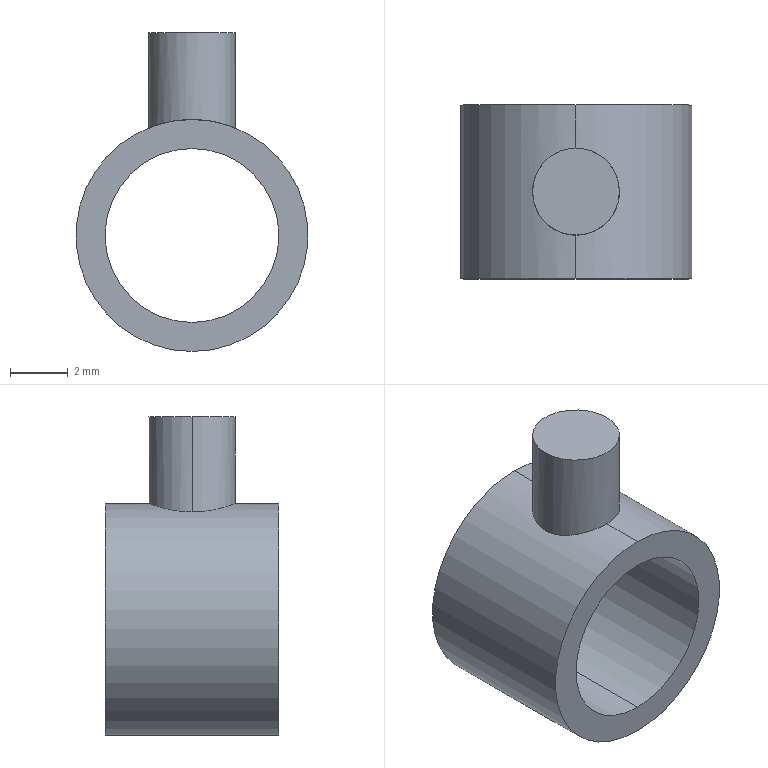Part | SolidWorks | features Extrusion 1, ICE 1 | 1 solid | 9 faces | box 8 x 6 x 11 mm | volume 153.659 mm3 | cylinder 6 | plane 3 | commonest cylinder face diameters 3 x2 6 x2 8 x2
STEP:
#1=CARTESIAN_POINT('',(0.,4.5,4.));
#2=VERTEX_POINT('',#1);
#3=CARTESIAN_POINT('',(-1.5,3.,3.708));
#4=VERTEX_POINT('',#3);
#5=CARTESIAN_POINT('',(0.,4.5,4.));
#6=CARTESIAN_POINT('',(-0.09889,4.5,4.));
#7=CARTESIAN_POINT('',(-0.1992,4.49,3.996));
#8=CARTESIAN_POINT('',(-0.3924,4.451,3.982));
#9=CARTESIAN_POINT('',(-0.4864,4.422,3.971));
#10=CARTESIAN_POINT('',(-0.6693,4.346,3.945));
#11=CARTESIAN_POINT('',(-0.7553,4.3,3.929));
#12=CARTESIAN_POINT('',(-0.9168,4.191,3.894));
#13=CARTESIAN_POINT('',(-0.9931,4.128,3.875));
#14=CARTESIAN_POINT('',(-1.131,3.991,3.838));
#15=CARTESIAN_POINT('',(-1.192,3.916,3.819));
#16=CARTESIAN_POINT('',(-1.3,3.754,3.783));
#17=CARTESIAN_POINT('',(-1.347,3.666,3.766));
#18=CARTESIAN_POINT('',(-1.46,3.396,3.725));
#19=CARTESIAN_POINT('',(-1.5,3.197,3.708));
#20=CARTESIAN_POINT('',(-1.5,3.,3.708));
#21=B_SPLINE_CURVE_WITH_KNOTS('',3,(#5,#6,#7,#8,#9,#10,#11,#12,#13,#14,#15,#16,#17,#18,#19,#20),.UNSPECIFIED.,.F.,.F.,(4,2,2,2,2,2,2,4),(0.002367,0.002663,0.002959,0.003255,0.00355,0.003846,0.004142,0.004733),.UNSPECIFIED.);
#22=EDGE_CURVE('',#2,#4,#21,.T.);
#23=ORIENTED_EDGE('',*,*,#22,.T.);
#24=CARTESIAN_POINT('',(-1.5,3.,7.));
#25=VERTEX_POINT('',#24);
#26=CARTESIAN_POINT('',(-1.5,3.,-4.001));
#27=DIRECTION('',(0.,0.,1.));
#28=VECTOR('',#27,1000.);
#29=LINE('',#26,#28);
#30=EDGE_CURVE('',#4,#25,#29,.T.);
#31=ORIENTED_EDGE('',*,*,#30,.T.);
#32=CARTESIAN_POINT('',(1.5,3.,7.));
#33=VERTEX_POINT('',#32);
#34=CARTESIAN_POINT('',(0.,3.,7.));
#35=DIRECTION('',(0.,0.,1.));
#36=DIRECTION('',(1.,0.,0.));
#37=AXIS2_PLACEMENT_3D('',#34,#35,#36);
#38=CIRCLE('',#37,1.5);
#39=EDGE_CURVE('',#33,#25,#38,.T.);
#40=ORIENTED_EDGE('',*,*,#39,.F.);
#41=CARTESIAN_POINT('',(1.5,3.,3.708));
#42=VERTEX_POINT('',#41);
#43=CARTESIAN_POINT('',(1.5,3.,-4.001));
#44=DIRECTION('',(0.,0.,1.));
#45=VECTOR('',#44,1000.);
#46=LINE('',#43,#45);
#47=EDGE_CURVE('',#42,#33,#46,.T.);
#48=ORIENTED_EDGE('',*,*,#47,.F.);
#49=CARTESIAN_POINT('',(1.5,3.,3.708));
#50=CARTESIAN_POINT('',(1.5,3.1,3.708));
#51=CARTESIAN_POINT('',(1.49,3.198,3.712));
#52=CARTESIAN_POINT('',(1.451,3.391,3.727));
#53=CARTESIAN_POINT('',(1.422,3.487,3.739));
#54=CARTESIAN_POINT('',(1.309,3.759,3.781));
#55=CARTESIAN_POINT('',(1.197,3.924,3.819));
#56=CARTESIAN_POINT('',(0.9232,4.198,3.895));
#57=CARTESIAN_POINT('',(0.7573,4.309,3.932));
#58=CARTESIAN_POINT('',(0.4867,4.422,3.971));
#59=CARTESIAN_POINT('',(0.3912,4.451,3.982));
#60=CARTESIAN_POINT('',(0.197,4.49,3.996));
#61=CARTESIAN_POINT('',(0.09895,4.5,4.));
#62=CARTESIAN_POINT('',(0.,4.5,4.));
#63=B_SPLINE_CURVE_WITH_KNOTS('',3,(#49,#50,#51,#52,#53,#54,#55,#56,#57,#58,#59,#60,#61,#62),.UNSPECIFIED.,.F.,.F.,(4,2,2,2,2,2,4),(0.,0.0002959,0.0005918,0.001184,0.001775,0.002071,0.002367),.UNSPECIFIED.);
#64=EDGE_CURVE('',#42,#2,#63,.T.);
#65=ORIENTED_EDGE('',*,*,#64,.T.);
#66=EDGE_LOOP('',(#23,#31,#40,#48,#65));
#67=FACE_OUTER_BOUND('',#66,.T.);
#68=CARTESIAN_POINT('',(0.,3.,-4.001));
#69=DIRECTION('',(0.,0.,1.));
#70=DIRECTION('',(1.,0.,0.));
#71=AXIS2_PLACEMENT_3D('',#68,#69,#70);
#72=CYLINDRICAL_SURFACE('',#71,1.5);
#73=ADVANCED_FACE('',(#67),#72,.T.);
#74=CARTESIAN_POINT('',(0.,6.,-3.));
#75=VERTEX_POINT('',#74);
#76=CARTESIAN_POINT('',(0.,6.,3.));
#77=VERTEX_POINT('',#76);
#78=CARTESIAN_POINT('',(0.,6.,0.));
#79=DIRECTION('',(0.,1.,0.));
#80=DIRECTION('',(0.,0.,1.));
#81=AXIS2_PLACEMENT_3D('',#78,#79,#80);
#82=CIRCLE('',#81,3.);
#83=EDGE_CURVE('',#75,#77,#82,.T.);
#84=ORIENTED_EDGE('',*,*,#83,.T.);
#85=CARTESIAN_POINT('',(0.,0.,3.));
#86=VERTEX_POINT('',#85);
#87=CARTESIAN_POINT('',(0.,6.,3.));
#88=DIRECTION('',(0.,-1.,0.));
#89=VECTOR('',#88,1000.);
#90=LINE('',#87,#89);
#91=EDGE_CURVE('',#77,#86,#90,.T.);
#92=ORIENTED_EDGE('',*,*,#91,.T.);
#93=CARTESIAN_POINT('',(0.,0.,-3.));
#94=VERTEX_POINT('',#93);
#95=CARTESIAN_POINT('',(0.,0.,0.));
#96=DIRECTION('',(0.,1.,0.));
#97=DIRECTION('',(0.,0.,1.));
#98=AXIS2_PLACEMENT_3D('',#95,#96,#97);
#99=CIRCLE('',#98,3.);
#100=EDGE_CURVE('',#94,#86,#99,.T.);
#101=ORIENTED_EDGE('',*,*,#100,.F.);
#102=CARTESIAN_POINT('',(0.,6.,-3.));
#103=DIRECTION('',(0.,-1.,0.));
#104=VECTOR('',#103,1000.);
#105=LINE('',#102,#104);
#106=EDGE_CURVE('',#75,#94,#105,.T.);
#107=ORIENTED_EDGE('',*,*,#106,.F.);
#108=EDGE_LOOP('',(#84,#92,#101,#107));
#109=FACE_OUTER_BOUND('',#108,.T.);
#110=CARTESIAN_POINT('',(0.,6.,0.));
#111=DIRECTION('',(0.,-1.,0.));
#112=DIRECTION('',(0.,0.,-1.));
#113=AXIS2_PLACEMENT_3D('',#110,#111,#112);
#114=CYLINDRICAL_SURFACE('',#113,3.);
#115=ADVANCED_FACE('',(#109),#114,.F.);
#116=CARTESIAN_POINT('',(0.,6.,4.));
#117=VERTEX_POINT('',#116);
#118=CARTESIAN_POINT('',(0.,6.,-4.));
#119=VERTEX_POINT('',#118);
#120=CARTESIAN_POINT('',(0.,6.,0.));
#121=DIRECTION('',(0.,1.,0.));
#122=DIRECTION('',(0.,0.,1.));
#123=AXIS2_PLACEMENT_3D('',#120,#121,#122);
#124=CIRCLE('',#123,4.);
#125=EDGE_CURVE('',#117,#119,#124,.T.);
#126=ORIENTED_EDGE('',*,*,#125,.F.);
#127=CARTESIAN_POINT('',(0.,6.,4.));
#128=DIRECTION('',(0.,-1.,0.));
#129=VECTOR('',#128,1000.);
#130=LINE('',#127,#129);
#131=EDGE_CURVE('',#117,#2,#130,.T.);
#132=ORIENTED_EDGE('',*,*,#131,.T.);
#133=ORIENTED_EDGE('',*,*,#64,.F.);
#134=CARTESIAN_POINT('',(0.,1.5,4.));
#135=VERTEX_POINT('',#134);
#136=CARTESIAN_POINT('',(0.,1.5,4.));
#137=CARTESIAN_POINT('',(0.1978,1.5,4.));
#138=CARTESIAN_POINT('',(0.3966,1.54,3.984));
#139=CARTESIAN_POINT('',(0.7582,1.691,3.932));
#140=CARTESIAN_POINT('',(0.9237,1.802,3.895));
#141=CARTESIAN_POINT('',(1.13,2.009,3.838));
#142=CARTESIAN_POINT('',(1.193,2.085,3.818));
#143=CARTESIAN_POINT('',(1.301,2.247,3.783));
#144=CARTESIAN_POINT('',(1.347,2.332,3.767));
#145=CARTESIAN_POINT('',(1.461,2.605,3.725));
#146=CARTESIAN_POINT('',(1.5,2.8,3.708));
#147=CARTESIAN_POINT('',(1.5,3.,3.708));
#148=B_SPLINE_CURVE_WITH_KNOTS('',3,(#136,#137,#138,#139,#140,#141,#142,#143,#144,#145,#146,#147),.UNSPECIFIED.,.F.,.F.,(4,2,2,2,2,4),(0.007099,0.00769,0.008282,0.008578,0.008874,0.009465),.UNSPECIFIED.);
#149=EDGE_CURVE('',#135,#42,#148,.T.);
#150=ORIENTED_EDGE('',*,*,#149,.F.);
#151=CARTESIAN_POINT('',(0.,0.,4.));
#152=VERTEX_POINT('',#151);
#153=CARTESIAN_POINT('',(0.,6.,4.));
#154=DIRECTION('',(0.,-1.,0.));
#155=VECTOR('',#154,1000.);
#156=LINE('',#153,#155);
#157=EDGE_CURVE('',#135,#152,#156,.T.);
#158=ORIENTED_EDGE('',*,*,#157,.T.);
#159=CARTESIAN_POINT('',(0.,0.,-4.));
#160=VERTEX_POINT('',#159);
#161=CARTESIAN_POINT('',(0.,0.,0.));
#162=DIRECTION('',(0.,1.,0.));
#163=DIRECTION('',(0.,0.,1.));
#164=AXIS2_PLACEMENT_3D('',#161,#162,#163);
#165=CIRCLE('',#164,4.);
#166=EDGE_CURVE('',#152,#160,#165,.T.);
#167=ORIENTED_EDGE('',*,*,#166,.T.);
#168=CARTESIAN_POINT('',(0.,6.,-4.));
#169=DIRECTION('',(0.,-1.,0.));
#170=VECTOR('',#169,1000.);
#171=LINE('',#168,#170);
#172=EDGE_CURVE('',#119,#160,#171,.T.);
#173=ORIENTED_EDGE('',*,*,#172,.F.);
#174=EDGE_LOOP('',(#126,#132,#133,#150,#158,#167,#173));
#175=FACE_OUTER_BOUND('',#174,.T.);
#176=CARTESIAN_POINT('',(0.,6.,0.));
#177=DIRECTION('',(0.,-1.,0.));
#178=DIRECTION('',(0.,0.,-1.));
#179=AXIS2_PLACEMENT_3D('',#176,#177,#178);
#180=CYLINDRICAL_SURFACE('',#179,4.);
#181=ADVANCED_FACE('',(#175),#180,.T.);
#182=CARTESIAN_POINT('',(0.,6.,0.));
#183=DIRECTION('',(0.,1.,0.));
#184=DIRECTION('',(0.,0.,1.));
#185=AXIS2_PLACEMENT_3D('',#182,#183,#184);
#186=CIRCLE('',#185,4.);
#187=EDGE_CURVE('',#119,#117,#186,.T.);
#188=ORIENTED_EDGE('',*,*,#187,.T.);
#189=ORIENTED_EDGE('',*,*,#125,.T.);
#190=EDGE_LOOP('',(#188,#189));
#191=FACE_OUTER_BOUND('',#190,.T.);
#192=ORIENTED_EDGE('',*,*,#83,.F.);
#193=CARTESIAN_POINT('',(0.,6.,0.));
#194=DIRECTION('',(0.,1.,0.));
#195=DIRECTION('',(0.,0.,1.));
#196=AXIS2_PLACEMENT_3D('',#193,#194,#195);
#197=CIRCLE('',#196,3.);
#198=EDGE_CURVE('',#77,#75,#197,.T.);
#199=ORIENTED_EDGE('',*,*,#198,.F.);
#200=EDGE_LOOP('',(#192,#199));
#201=FACE_BOUND('',#200,.T.);
#202=CARTESIAN_POINT('',(0.,6.,0.));
#203=DIRECTION('',(0.,1.,0.));
#204=DIRECTION('',(0.,0.,1.));
#205=AXIS2_PLACEMENT_3D('',#202,#203,#204);
#206=PLANE('',#205);
#207=ADVANCED_FACE('',(#191,#201),#206,.T.);
#208=CARTESIAN_POINT('',(0.,0.,0.));
#209=DIRECTION('',(0.,1.,0.));
#210=DIRECTION('',(0.,0.,1.));
#211=AXIS2_PLACEMENT_3D('',#208,#209,#210);
#212=CIRCLE('',#211,4.);
#213=EDGE_CURVE('',#160,#152,#212,.T.);
#214=ORIENTED_EDGE('',*,*,#213,.F.);
#215=ORIENTED_EDGE('',*,*,#166,.F.);
#216=EDGE_LOOP('',(#214,#215));
#217=FACE_OUTER_BOUND('',#216,.T.);
#218=ORIENTED_EDGE('',*,*,#100,.T.);
#219=CARTESIAN_POINT('',(0.,0.,0.));
#220=DIRECTION('',(0.,1.,0.));
#221=DIRECTION('',(0.,0.,1.));
#222=AXIS2_PLACEMENT_3D('',#219,#220,#221);
#223=CIRCLE('',#222,3.);
#224=EDGE_CURVE('',#86,#94,#223,.T.);
#225=ORIENTED_EDGE('',*,*,#224,.T.);
#226=EDGE_LOOP('',(#218,#225));
#227=FACE_BOUND('',#226,.T.);
#228=CARTESIAN_POINT('',(0.,0.,0.));
#229=DIRECTION('',(0.,1.,0.));
#230=DIRECTION('',(0.,0.,1.));
#231=AXIS2_PLACEMENT_3D('',#228,#229,#230);
#232=PLANE('',#231);
#233=ADVANCED_FACE('',(#217,#227),#232,.F.);
#234=ORIENTED_EDGE('',*,*,#131,.F.);
#235=ORIENTED_EDGE('',*,*,#187,.F.);
#236=ORIENTED_EDGE('',*,*,#172,.T.);
#237=ORIENTED_EDGE('',*,*,#213,.T.);
#238=ORIENTED_EDGE('',*,*,#157,.F.);
#239=CARTESIAN_POINT('',(-1.5,3.,3.708));
#240=CARTESIAN_POINT('',(-1.5,2.803,3.708));
#241=CARTESIAN_POINT('',(-1.46,2.604,3.725));
#242=CARTESIAN_POINT('',(-1.347,2.333,3.767));
#243=CARTESIAN_POINT('',(-1.3,2.245,3.783));
#244=CARTESIAN_POINT('',(-1.192,2.084,3.819));
#245=CARTESIAN_POINT('',(-1.13,2.009,3.838));
#246=CARTESIAN_POINT('',(-0.9219,1.801,3.895));
#247=CARTESIAN_POINT('',(-0.7585,1.691,3.932));
#248=CARTESIAN_POINT('',(-0.486,1.577,3.971));
#249=CARTESIAN_POINT('',(-0.3923,1.549,3.982));
#250=CARTESIAN_POINT('',(-0.1993,1.51,3.996));
#251=CARTESIAN_POINT('',(-0.09883,1.5,4.));
#252=CARTESIAN_POINT('',(0.,1.5,4.));
#253=B_SPLINE_CURVE_WITH_KNOTS('',3,(#239,#240,#241,#242,#243,#244,#245,#246,#247,#248,#249,#250,#251,#252),.UNSPECIFIED.,.F.,.F.,(4,2,2,2,2,2,4),(0.004733,0.005325,0.00562,0.005916,0.006507,0.006803,0.007099),.UNSPECIFIED.);
#254=EDGE_CURVE('',#4,#135,#253,.T.);
#255=ORIENTED_EDGE('',*,*,#254,.F.);
#256=ORIENTED_EDGE('',*,*,#22,.F.);
#257=EDGE_LOOP('',(#234,#235,#236,#237,#238,#255,#256));
#258=FACE_OUTER_BOUND('',#257,.T.);
#259=CARTESIAN_POINT('',(0.,6.,0.));
#260=DIRECTION('',(0.,-1.,0.));
#261=DIRECTION('',(0.,0.,-1.));
#262=AXIS2_PLACEMENT_3D('',#259,#260,#261);
#263=CYLINDRICAL_SURFACE('',#262,4.);
#264=ADVANCED_FACE('',(#258),#263,.T.);
#265=ORIENTED_EDGE('',*,*,#91,.F.);
#266=ORIENTED_EDGE('',*,*,#198,.T.);
#267=ORIENTED_EDGE('',*,*,#106,.T.);
#268=ORIENTED_EDGE('',*,*,#224,.F.);
#269=EDGE_LOOP('',(#265,#266,#267,#268));
#270=FACE_OUTER_BOUND('',#269,.T.);
#271=CARTESIAN_POINT('',(0.,6.,0.));
#272=DIRECTION('',(0.,-1.,0.));
#273=DIRECTION('',(0.,0.,-1.));
#274=AXIS2_PLACEMENT_3D('',#271,#272,#273);
#275=CYLINDRICAL_SURFACE('',#274,3.);
#276=ADVANCED_FACE('',(#270),#275,.F.);
#277=ORIENTED_EDGE('',*,*,#39,.T.);
#278=CARTESIAN_POINT('',(0.,3.,7.));
#279=DIRECTION('',(0.,0.,1.));
#280=DIRECTION('',(1.,0.,0.));
#281=AXIS2_PLACEMENT_3D('',#278,#279,#280);
#282=CIRCLE('',#281,1.5);
#283=EDGE_CURVE('',#25,#33,#282,.T.);
#284=ORIENTED_EDGE('',*,*,#283,.T.);
#285=EDGE_LOOP('',(#277,#284));
#286=FACE_OUTER_BOUND('',#285,.T.);
#287=CARTESIAN_POINT('',(0.,3.,7.));
#288=DIRECTION('',(0.,0.,1.));
#289=DIRECTION('',(1.,0.,0.));
#290=AXIS2_PLACEMENT_3D('',#287,#288,#289);
#291=PLANE('',#290);
#292=ADVANCED_FACE('',(#286),#291,.T.);
#293=ORIENTED_EDGE('',*,*,#30,.F.);
#294=ORIENTED_EDGE('',*,*,#254,.T.);
#295=ORIENTED_EDGE('',*,*,#149,.T.);
#296=ORIENTED_EDGE('',*,*,#47,.T.);
#297=ORIENTED_EDGE('',*,*,#283,.F.);
#298=EDGE_LOOP('',(#293,#294,#295,#296,#297));
#299=FACE_OUTER_BOUND('',#298,.T.);
#300=CARTESIAN_POINT('',(0.,3.,-4.001));
#301=DIRECTION('',(0.,0.,1.));
#302=DIRECTION('',(1.,0.,0.));
#303=AXIS2_PLACEMENT_3D('',#300,#301,#302);
#304=CYLINDRICAL_SURFACE('',#303,1.5);
#305=ADVANCED_FACE('',(#299),#304,.T.);
#306=CLOSED_SHELL('',(#73,#115,#181,#207,#233,#264,#276,#292,#305));
#307=MANIFOLD_SOLID_BREP('',#306);
#308=CARTESIAN_POINT('',(0.,0.,0.));
#309=DIRECTION('',(0.,0.,1.));
#310=DIRECTION('',(1.,0.,0.));
#311=AXIS2_PLACEMENT_3D('',#308,#309,#310);
#312=(LENGTH_UNIT()NAMED_UNIT(*)SI_UNIT(.MILLI.,.METRE.));
#313=UNCERTAINTY_MEASURE_WITH_UNIT(LENGTH_MEASURE(0.00001),#312,'','');
#314=(NAMED_UNIT(*)PLANE_ANGLE_UNIT()SI_UNIT($,.RADIAN.));
#315=(NAMED_UNIT(*)SI_UNIT($,.STERADIAN.)SOLID_ANGLE_UNIT());
#316=(GEOMETRIC_REPRESENTATION_CONTEXT(3)GLOBAL_UNCERTAINTY_ASSIGNED_CONTEXT((#313))GLOBAL_UNIT_ASSIGNED_CONTEXT((#312,#314,#315))REPRESENTATION_CONTEXT('',''));
#317=ADVANCED_BREP_SHAPE_REPRESENTATION('',(#307,#311),#316);